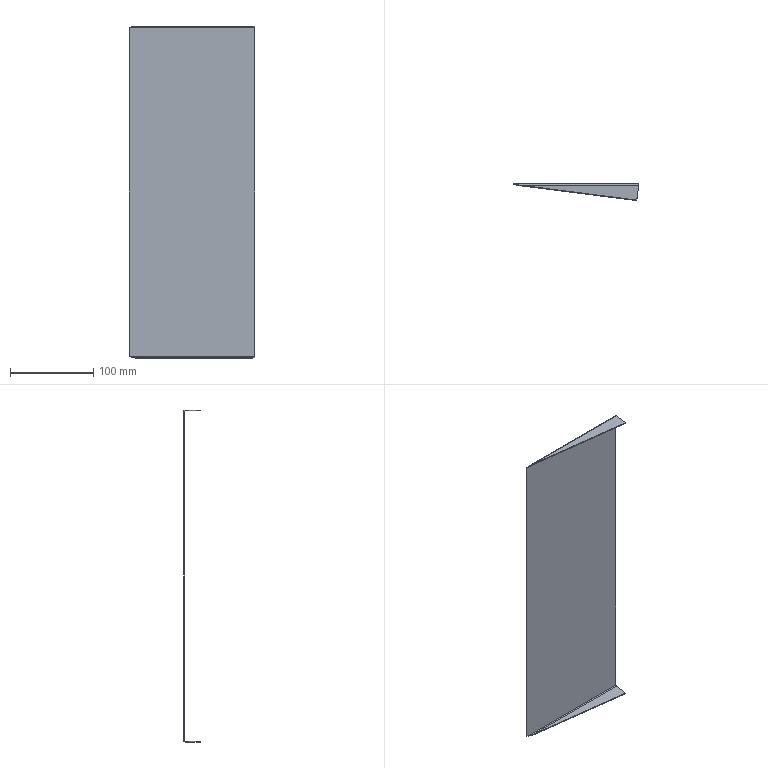Part | SolidWorks | features EdgeFlange 1, FlatPattern 1, MirrorPattern 1, SMBaseFlange 1, SheetMetal 1 | 1 solid | 20 faces | box 151 x 20 x 399 mm | volume 62913 mm3 | plane 12 | spline 4 | cylinder 4 | commonest cylinder face diameters 2 x2 4 x2
STEP:
#1=CARTESIAN_POINT('',(0.,-1.,-197.5));
#2=VERTEX_POINT('',#1);
#3=CARTESIAN_POINT('',(-151.,-1.,-197.5));
#4=VERTEX_POINT('',#3);
#5=CARTESIAN_POINT('',(0.,-1.,-197.5));
#6=DIRECTION('',(-1.,0.,0.));
#7=VECTOR('',#6,1000.);
#8=LINE('',#5,#7);
#9=EDGE_CURVE('',#2,#4,#8,.T.);
#10=ORIENTED_EDGE('',*,*,#9,.F.);
#11=CARTESIAN_POINT('',(0.,-1.,197.5));
#12=VERTEX_POINT('',#11);
#13=CARTESIAN_POINT('',(0.,-1.,199.5));
#14=DIRECTION('',(0.,0.,-1.));
#15=VECTOR('',#14,1000.);
#16=LINE('',#13,#15);
#17=EDGE_CURVE('',#12,#2,#16,.T.);
#18=ORIENTED_EDGE('',*,*,#17,.F.);
#19=CARTESIAN_POINT('',(-151.,-1.,197.5));
#20=VERTEX_POINT('',#19);
#21=CARTESIAN_POINT('',(-151.,-1.,197.5));
#22=DIRECTION('',(1.,0.,0.));
#23=VECTOR('',#22,1000.);
#24=LINE('',#21,#23);
#25=EDGE_CURVE('',#20,#12,#24,.T.);
#26=ORIENTED_EDGE('',*,*,#25,.F.);
#27=CARTESIAN_POINT('',(-151.,-1.,199.5));
#28=DIRECTION('',(0.,0.,-1.));
#29=VECTOR('',#28,1000.);
#30=LINE('',#27,#29);
#31=EDGE_CURVE('',#20,#4,#30,.T.);
#32=ORIENTED_EDGE('',*,*,#31,.T.);
#33=EDGE_LOOP('',(#10,#18,#26,#32));
#34=FACE_OUTER_BOUND('',#33,.T.);
#35=CARTESIAN_POINT('',(-151.,-1.,199.5));
#36=DIRECTION('',(0.,1.,0.));
#37=DIRECTION('',(0.,0.,1.));
#38=AXIS2_PLACEMENT_3D('',#35,#36,#37);
#39=PLANE('',#38);
#40=ADVANCED_FACE('',(#34),#39,.F.);
#41=CARTESIAN_POINT('',(0.,0.,197.5));
#42=VERTEX_POINT('',#41);
#43=CARTESIAN_POINT('',(0.,0.,-197.5));
#44=VERTEX_POINT('',#43);
#45=CARTESIAN_POINT('',(0.,0.,199.5));
#46=DIRECTION('',(0.,0.,-1.));
#47=VECTOR('',#46,1000.);
#48=LINE('',#45,#47);
#49=EDGE_CURVE('',#42,#44,#48,.T.);
#50=ORIENTED_EDGE('',*,*,#49,.T.);
#51=CARTESIAN_POINT('',(-151.,0.,-197.5));
#52=VERTEX_POINT('',#51);
#53=CARTESIAN_POINT('',(0.,0.,-197.5));
#54=DIRECTION('',(-1.,0.,0.));
#55=VECTOR('',#54,1000.);
#56=LINE('',#53,#55);
#57=EDGE_CURVE('',#44,#52,#56,.T.);
#58=ORIENTED_EDGE('',*,*,#57,.T.);
#59=CARTESIAN_POINT('',(-151.,0.,197.5));
#60=VERTEX_POINT('',#59);
#61=CARTESIAN_POINT('',(-151.,0.,199.5));
#62=DIRECTION('',(0.,0.,-1.));
#63=VECTOR('',#62,1000.);
#64=LINE('',#61,#63);
#65=EDGE_CURVE('',#60,#52,#64,.T.);
#66=ORIENTED_EDGE('',*,*,#65,.F.);
#67=CARTESIAN_POINT('',(-151.,0.,197.5));
#68=DIRECTION('',(1.,0.,0.));
#69=VECTOR('',#68,1000.);
#70=LINE('',#67,#69);
#71=EDGE_CURVE('',#60,#42,#70,.T.);
#72=ORIENTED_EDGE('',*,*,#71,.T.);
#73=EDGE_LOOP('',(#50,#58,#66,#72));
#74=FACE_OUTER_BOUND('',#73,.T.);
#75=CARTESIAN_POINT('',(-151.,0.,199.5));
#76=DIRECTION('',(0.,1.,0.));
#77=DIRECTION('',(0.,0.,1.));
#78=AXIS2_PLACEMENT_3D('',#75,#76,#77);
#79=PLANE('',#78);
#80=ADVANCED_FACE('',(#74),#79,.T.);
#81=ORIENTED_EDGE('',*,*,#17,.T.);
#82=CARTESIAN_POINT('',(0.,-1.,-197.5));
#83=DIRECTION('',(0.,1.,0.));
#84=VECTOR('',#83,1000.);
#85=LINE('',#82,#84);
#86=EDGE_CURVE('',#2,#44,#85,.T.);
#87=ORIENTED_EDGE('',*,*,#86,.T.);
#88=ORIENTED_EDGE('',*,*,#49,.F.);
#89=CARTESIAN_POINT('',(0.,-1.,197.5));
#90=DIRECTION('',(0.,1.,0.));
#91=VECTOR('',#90,1000.);
#92=LINE('',#89,#91);
#93=EDGE_CURVE('',#12,#42,#92,.T.);
#94=ORIENTED_EDGE('',*,*,#93,.F.);
#95=EDGE_LOOP('',(#81,#87,#88,#94));
#96=FACE_OUTER_BOUND('',#95,.T.);
#97=CARTESIAN_POINT('',(0.,0.,199.5));
#98=DIRECTION('',(1.,0.,0.));
#99=DIRECTION('',(0.,0.,-1.));
#100=AXIS2_PLACEMENT_3D('',#97,#98,#99);
#101=PLANE('',#100);
#102=ADVANCED_FACE('',(#96),#101,.T.);
#103=CARTESIAN_POINT('',(-151.,-1.,-197.5));
#104=DIRECTION('',(0.,1.,0.));
#105=VECTOR('',#104,1000.);
#106=LINE('',#103,#105);
#107=EDGE_CURVE('',#4,#52,#106,.T.);
#108=ORIENTED_EDGE('',*,*,#107,.F.);
#109=ORIENTED_EDGE('',*,*,#31,.F.);
#110=CARTESIAN_POINT('',(-151.,-1.,197.5));
#111=DIRECTION('',(0.,1.,0.));
#112=VECTOR('',#111,1000.);
#113=LINE('',#110,#112);
#114=EDGE_CURVE('',#20,#60,#113,.T.);
#115=ORIENTED_EDGE('',*,*,#114,.T.);
#116=ORIENTED_EDGE('',*,*,#65,.T.);
#117=EDGE_LOOP('',(#108,#109,#115,#116));
#118=FACE_OUTER_BOUND('',#117,.T.);
#119=CARTESIAN_POINT('',(-151.,-1.,199.5));
#120=DIRECTION('',(-1.,0.,0.));
#121=DIRECTION('',(0.,0.,1.));
#122=AXIS2_PLACEMENT_3D('',#119,#120,#121);
#123=PLANE('',#122);
#124=ADVANCED_FACE('',(#118),#123,.T.);
#125=CARTESIAN_POINT('',(-0.1279,-2.,198.5));
#126=VERTEX_POINT('',#125);
#127=CARTESIAN_POINT('',(-0.1279,-2.,199.5));
#128=VERTEX_POINT('',#127);
#129=CARTESIAN_POINT('',(-0.1279,-2.,199.5));
#130=DIRECTION('',(0.,0.,1.));
#131=VECTOR('',#130,1000.);
#132=LINE('',#129,#131);
#133=EDGE_CURVE('',#126,#128,#132,.T.);
#134=ORIENTED_EDGE('',*,*,#133,.F.);
#135=CARTESIAN_POINT('',(0.,-1.,197.5));
#136=CARTESIAN_POINT('',(-0.02131,-1.,197.762));
#137=CARTESIAN_POINT('',(-0.04263,-1.108,198.022));
#138=CARTESIAN_POINT('',(-0.08526,-1.478,198.392));
#139=CARTESIAN_POINT('',(-0.1066,-1.738,198.5));
#140=CARTESIAN_POINT('',(-0.1279,-2.,198.5));
#141=B_SPLINE_CURVE_WITH_KNOTS('',3,(#135,#136,#137,#138,#139,#140),.UNSPECIFIED.,.F.,.F.,(4,2,4),(0.,0.5,1.),.UNSPECIFIED.);
#142=EDGE_CURVE('',#12,#126,#141,.T.);
#143=ORIENTED_EDGE('',*,*,#142,.F.);
#144=ORIENTED_EDGE('',*,*,#93,.T.);
#145=CARTESIAN_POINT('',(0.,0.,197.5));
#146=CARTESIAN_POINT('',(-0.01066,0.,197.762));
#147=CARTESIAN_POINT('',(-0.02131,-0.05205,198.023));
#148=CARTESIAN_POINT('',(-0.04263,-0.2524,198.507));
#149=CARTESIAN_POINT('',(-0.05329,-0.4007,198.729));
#150=CARTESIAN_POINT('',(-0.0746,-0.7709,199.099));
#151=CARTESIAN_POINT('',(-0.08526,-0.9928,199.248));
#152=CARTESIAN_POINT('',(-0.1066,-1.477,199.448));
#153=CARTESIAN_POINT('',(-0.1172,-1.738,199.5));
#154=CARTESIAN_POINT('',(-0.1279,-2.,199.5));
#155=B_SPLINE_CURVE_WITH_KNOTS('',3,(#145,#146,#147,#148,#149,#150,#151,#152,#153,#154),.UNSPECIFIED.,.F.,.F.,(4,2,2,2,4),(0.,0.25,0.5,0.75,1.),.UNSPECIFIED.);
#156=EDGE_CURVE('',#42,#128,#155,.T.);
#157=ORIENTED_EDGE('',*,*,#156,.T.);
#158=EDGE_LOOP('',(#134,#143,#144,#157));
#159=FACE_OUTER_BOUND('',#158,.T.);
#160=CARTESIAN_POINT('',(0.,0.01,197.5));
#161=CARTESIAN_POINT('',(-0.01066,0.01,197.763));
#162=CARTESIAN_POINT('',(-0.02131,-0.04231,198.026));
#163=CARTESIAN_POINT('',(-0.04263,-0.2437,198.512));
#164=CARTESIAN_POINT('',(-0.05329,-0.3927,198.735));
#165=CARTESIAN_POINT('',(-0.0746,-0.7648,199.107));
#166=CARTESIAN_POINT('',(-0.08526,-0.9877,199.256));
#167=CARTESIAN_POINT('',(-0.1066,-1.474,199.458));
#168=CARTESIAN_POINT('',(-0.1172,-1.737,199.51));
#169=CARTESIAN_POINT('',(-0.1279,-2.,199.51));
#170=CARTESIAN_POINT('',(0.,0.,197.5));
#171=CARTESIAN_POINT('',(-0.01066,0.,197.762));
#172=CARTESIAN_POINT('',(-0.02131,-0.05205,198.023));
#173=CARTESIAN_POINT('',(-0.04263,-0.2524,198.507));
#174=CARTESIAN_POINT('',(-0.05329,-0.4007,198.729));
#175=CARTESIAN_POINT('',(-0.0746,-0.7709,199.099));
#176=CARTESIAN_POINT('',(-0.08526,-0.9928,199.248));
#177=CARTESIAN_POINT('',(-0.1066,-1.477,199.448));
#178=CARTESIAN_POINT('',(-0.1172,-1.738,199.5));
#179=CARTESIAN_POINT('',(-0.1279,-2.,199.5));
#180=CARTESIAN_POINT('',(0.,-1.,197.5));
#181=CARTESIAN_POINT('',(-0.01066,-1.,197.631));
#182=CARTESIAN_POINT('',(-0.02131,-1.026,197.762));
#183=CARTESIAN_POINT('',(-0.04263,-1.126,198.004));
#184=CARTESIAN_POINT('',(-0.05329,-1.2,198.115));
#185=CARTESIAN_POINT('',(-0.0746,-1.385,198.3));
#186=CARTESIAN_POINT('',(-0.08526,-1.496,198.374));
#187=CARTESIAN_POINT('',(-0.1066,-1.738,198.474));
#188=CARTESIAN_POINT('',(-0.1172,-1.869,198.5));
#189=CARTESIAN_POINT('',(-0.1279,-2.,198.5));
#190=CARTESIAN_POINT('',(0.,-1.01,197.5));
#191=CARTESIAN_POINT('',(-0.01066,-1.01,197.63));
#192=CARTESIAN_POINT('',(-0.02131,-1.036,197.759));
#193=CARTESIAN_POINT('',(-0.04263,-1.135,197.999));
#194=CARTESIAN_POINT('',(-0.05329,-1.208,198.108));
#195=CARTESIAN_POINT('',(-0.0746,-1.392,198.292));
#196=CARTESIAN_POINT('',(-0.08526,-1.501,198.365));
#197=CARTESIAN_POINT('',(-0.1066,-1.741,198.464));
#198=CARTESIAN_POINT('',(-0.1172,-1.87,198.49));
#199=CARTESIAN_POINT('',(-0.1279,-2.,198.49));
#200=B_SPLINE_SURFACE_WITH_KNOTS('',1,3,((#160,#161,#162,#163,#164,#165,#166,#167,#168,#169),(#170,#171,#172,#173,#174,#175,#176,#177,#178,#179),(#180,#181,#182,#183,#184,#185,#186,#187,#188,#189),(#190,#191,#192,#193,#194,#195,#196,#197,#198,#199)),.UNSPECIFIED.,.F.,.F.,.F.,(2,1,1,2),(4,2,2,2,4),(-0.01,0.,1.,1.01),(0.,0.25,0.5,0.75,1.),.UNSPECIFIED.);
#201=ADVANCED_FACE('',(#159),#200,.F.);
#202=CARTESIAN_POINT('',(-143.181,-2.,198.5));
#203=VERTEX_POINT('',#202);
#204=CARTESIAN_POINT('',(-143.181,-2.,198.5));
#205=CARTESIAN_POINT('',(-144.485,-1.738,198.5));
#206=CARTESIAN_POINT('',(-145.788,-1.478,198.392));
#207=CARTESIAN_POINT('',(-148.398,-1.107,198.021));
#208=CARTESIAN_POINT('',(-149.695,-1.,197.762));
#209=CARTESIAN_POINT('',(-151.,-1.,197.5));
#210=B_SPLINE_CURVE_WITH_KNOTS('',3,(#204,#205,#206,#207,#208,#209),.UNSPECIFIED.,.F.,.F.,(4,2,4),(0.,0.00399,0.007979),.UNSPECIFIED.);
#211=EDGE_CURVE('',#203,#20,#210,.T.);
#212=ORIENTED_EDGE('',*,*,#211,.F.);
#213=CARTESIAN_POINT('',(-143.181,-2.,199.5));
#214=VERTEX_POINT('',#213);
#215=CARTESIAN_POINT('',(-143.181,-2.,198.5));
#216=DIRECTION('',(0.,0.,1.));
#217=VECTOR('',#216,1000.);
#218=LINE('',#215,#217);
#219=EDGE_CURVE('',#203,#214,#218,.T.);
#220=ORIENTED_EDGE('',*,*,#219,.T.);
#221=CARTESIAN_POINT('',(-143.181,-2.,199.5));
#222=CARTESIAN_POINT('',(-143.835,-1.737,199.5));
#223=CARTESIAN_POINT('',(-144.487,-1.475,199.448));
#224=CARTESIAN_POINT('',(-145.794,-0.9902,199.246));
#225=CARTESIAN_POINT('',(-146.442,-0.7701,199.098));
#226=CARTESIAN_POINT('',(-147.738,-0.4018,198.73));
#227=CARTESIAN_POINT('',(-148.388,-0.2535,198.509));
#228=CARTESIAN_POINT('',(-149.695,-0.05212,198.024));
#229=CARTESIAN_POINT('',(-150.346,0.,197.763));
#230=CARTESIAN_POINT('',(-151.,0.,197.5));
#231=B_SPLINE_CURVE_WITH_KNOTS('',3,(#221,#222,#223,#224,#225,#226,#227,#228,#229,#230),.UNSPECIFIED.,.F.,.F.,(4,2,2,2,4),(0.,0.00211,0.004221,0.006331,0.008441),.UNSPECIFIED.);
#232=EDGE_CURVE('',#214,#60,#231,.T.);
#233=ORIENTED_EDGE('',*,*,#232,.T.);
#234=ORIENTED_EDGE('',*,*,#114,.F.);
#235=EDGE_LOOP('',(#212,#220,#233,#234));
#236=FACE_OUTER_BOUND('',#235,.T.);
#237=CARTESIAN_POINT('',(-143.181,-2.,199.51));
#238=CARTESIAN_POINT('',(-143.832,-1.737,199.51));
#239=CARTESIAN_POINT('',(-144.484,-1.474,199.458));
#240=CARTESIAN_POINT('',(-145.787,-0.9877,199.256));
#241=CARTESIAN_POINT('',(-146.439,-0.7648,199.107));
#242=CARTESIAN_POINT('',(-147.742,-0.3927,198.735));
#243=CARTESIAN_POINT('',(-148.394,-0.2437,198.512));
#244=CARTESIAN_POINT('',(-149.697,-0.04231,198.026));
#245=CARTESIAN_POINT('',(-150.348,0.01,197.763));
#246=CARTESIAN_POINT('',(-151.,0.01,197.5));
#247=CARTESIAN_POINT('',(-143.181,-2.,199.5));
#248=CARTESIAN_POINT('',(-143.832,-1.738,199.5));
#249=CARTESIAN_POINT('',(-144.484,-1.477,199.448));
#250=CARTESIAN_POINT('',(-145.787,-0.9928,199.248));
#251=CARTESIAN_POINT('',(-146.439,-0.7709,199.099));
#252=CARTESIAN_POINT('',(-147.742,-0.4007,198.729));
#253=CARTESIAN_POINT('',(-148.394,-0.2524,198.507));
#254=CARTESIAN_POINT('',(-149.697,-0.05205,198.023));
#255=CARTESIAN_POINT('',(-150.348,0.,197.762));
#256=CARTESIAN_POINT('',(-151.,0.,197.5));
#257=CARTESIAN_POINT('',(-143.181,-2.,198.5));
#258=CARTESIAN_POINT('',(-143.832,-1.869,198.5));
#259=CARTESIAN_POINT('',(-144.484,-1.738,198.474));
#260=CARTESIAN_POINT('',(-145.787,-1.496,198.374));
#261=CARTESIAN_POINT('',(-146.439,-1.385,198.3));
#262=CARTESIAN_POINT('',(-147.742,-1.2,198.115));
#263=CARTESIAN_POINT('',(-148.394,-1.126,198.004));
#264=CARTESIAN_POINT('',(-149.697,-1.026,197.762));
#265=CARTESIAN_POINT('',(-150.348,-1.,197.631));
#266=CARTESIAN_POINT('',(-151.,-1.,197.5));
#267=CARTESIAN_POINT('',(-143.181,-2.,198.49));
#268=CARTESIAN_POINT('',(-143.832,-1.87,198.49));
#269=CARTESIAN_POINT('',(-144.484,-1.741,198.464));
#270=CARTESIAN_POINT('',(-145.787,-1.501,198.365));
#271=CARTESIAN_POINT('',(-146.439,-1.392,198.292));
#272=CARTESIAN_POINT('',(-147.742,-1.208,198.108));
#273=CARTESIAN_POINT('',(-148.394,-1.135,197.999));
#274=CARTESIAN_POINT('',(-149.697,-1.036,197.759));
#275=CARTESIAN_POINT('',(-150.348,-1.01,197.63));
#276=CARTESIAN_POINT('',(-151.,-1.01,197.5));
#277=B_SPLINE_SURFACE_WITH_KNOTS('',1,3,((#237,#238,#239,#240,#241,#242,#243,#244,#245,#246),(#247,#248,#249,#250,#251,#252,#253,#254,#255,#256),(#257,#258,#259,#260,#261,#262,#263,#264,#265,#266),(#267,#268,#269,#270,#271,#272,#273,#274,#275,#276)),.UNSPECIFIED.,.F.,.F.,.F.,(2,1,1,2),(4,2,2,2,4),(-0.01,0.,1.,1.01),(0.,0.25,0.5,0.75,1.),.UNSPECIFIED.);
#278=ADVANCED_FACE('',(#236),#277,.F.);
#279=ORIENTED_EDGE('',*,*,#71,.F.);
#280=ORIENTED_EDGE('',*,*,#232,.F.);
#281=CARTESIAN_POINT('',(-0.1279,-2.,199.5));
#282=DIRECTION('',(1.,0.,0.));
#283=VECTOR('',#282,1000.);
#284=LINE('',#281,#283);
#285=EDGE_CURVE('',#214,#128,#284,.T.);
#286=ORIENTED_EDGE('',*,*,#285,.T.);
#287=ORIENTED_EDGE('',*,*,#156,.F.);
#288=EDGE_LOOP('',(#279,#280,#286,#287));
#289=FACE_OUTER_BOUND('',#288,.T.);
#290=CARTESIAN_POINT('',(-151.,-2.,197.5));
#291=DIRECTION('',(-1.,0.,0.));
#292=DIRECTION('',(0.,0.,1.));
#293=AXIS2_PLACEMENT_3D('',#290,#291,#292);
#294=CYLINDRICAL_SURFACE('',#293,2.);
#295=ADVANCED_FACE('',(#289),#294,.T.);
#296=ORIENTED_EDGE('',*,*,#25,.T.);
#297=ORIENTED_EDGE('',*,*,#142,.T.);
#298=CARTESIAN_POINT('',(-0.1279,-2.,198.5));
#299=DIRECTION('',(-1.,0.,0.));
#300=VECTOR('',#299,1000.);
#301=LINE('',#298,#300);
#302=EDGE_CURVE('',#126,#203,#301,.T.);
#303=ORIENTED_EDGE('',*,*,#302,.T.);
#304=ORIENTED_EDGE('',*,*,#211,.T.);
#305=EDGE_LOOP('',(#296,#297,#303,#304));
#306=FACE_OUTER_BOUND('',#305,.T.);
#307=CARTESIAN_POINT('',(-151.,-2.,197.5));
#308=DIRECTION('',(-1.,0.,0.));
#309=DIRECTION('',(0.,0.,1.));
#310=AXIS2_PLACEMENT_3D('',#307,#308,#309);
#311=CYLINDRICAL_SURFACE('',#310,1.);
#312=ADVANCED_FACE('',(#306),#311,.F.);
#313=CARTESIAN_POINT('',(-2.43,-20.,199.5));
#314=VERTEX_POINT('',#313);
#315=CARTESIAN_POINT('',(-151.,-1.,199.5));
#316=DIRECTION('',(-0.9919,0.1269,0.));
#317=VECTOR('',#316,1000.);
#318=LINE('',#315,#317);
#319=EDGE_CURVE('',#314,#214,#318,.T.);
#320=ORIENTED_EDGE('',*,*,#319,.T.);
#321=ORIENTED_EDGE('',*,*,#219,.F.);
#322=CARTESIAN_POINT('',(-2.43,-20.,198.5));
#323=VERTEX_POINT('',#322);
#324=CARTESIAN_POINT('',(-2.556,-19.984,198.5));
#325=DIRECTION('',(-0.9919,0.1269,0.));
#326=VECTOR('',#325,1000.);
#327=LINE('',#324,#326);
#328=EDGE_CURVE('',#323,#203,#327,.T.);
#329=ORIENTED_EDGE('',*,*,#328,.F.);
#330=CARTESIAN_POINT('',(-2.43,-20.,199.5));
#331=DIRECTION('',(0.,0.,-1.));
#332=VECTOR('',#331,1000.);
#333=LINE('',#330,#332);
#334=EDGE_CURVE('',#314,#323,#333,.T.);
#335=ORIENTED_EDGE('',*,*,#334,.F.);
#336=EDGE_LOOP('',(#320,#321,#329,#335));
#337=FACE_OUTER_BOUND('',#336,.T.);
#338=CARTESIAN_POINT('',(-151.,-1.,199.5));
#339=DIRECTION('',(-0.1269,-0.9919,0.));
#340=DIRECTION('',(0.9919,-0.1269,0.));
#341=AXIS2_PLACEMENT_3D('',#338,#339,#340);
#342=PLANE('',#341);
#343=ADVANCED_FACE('',(#337),#342,.T.);
#344=CARTESIAN_POINT('',(0.1258,-0.01609,198.5));
#345=DIRECTION('',(-0.1269,-0.9919,0.));
#346=VECTOR('',#345,1000.);
#347=LINE('',#344,#346);
#348=EDGE_CURVE('',#126,#323,#347,.T.);
#349=ORIENTED_EDGE('',*,*,#348,.F.);
#350=ORIENTED_EDGE('',*,*,#133,.T.);
#351=CARTESIAN_POINT('',(-2.43,-20.,199.5));
#352=DIRECTION('',(-0.1269,-0.9919,0.));
#353=VECTOR('',#352,1000.);
#354=LINE('',#351,#353);
#355=EDGE_CURVE('',#128,#314,#354,.T.);
#356=ORIENTED_EDGE('',*,*,#355,.T.);
#357=ORIENTED_EDGE('',*,*,#334,.T.);
#358=EDGE_LOOP('',(#349,#350,#356,#357));
#359=FACE_OUTER_BOUND('',#358,.T.);
#360=CARTESIAN_POINT('',(-2.43,-20.,199.5));
#361=DIRECTION('',(0.9919,-0.1269,0.));
#362=DIRECTION('',(0.1269,0.9919,0.));
#363=AXIS2_PLACEMENT_3D('',#360,#361,#362);
#364=PLANE('',#363);
#365=ADVANCED_FACE('',(#359),#364,.T.);
#366=ORIENTED_EDGE('',*,*,#285,.F.);
#367=ORIENTED_EDGE('',*,*,#319,.F.);
#368=ORIENTED_EDGE('',*,*,#355,.F.);
#369=EDGE_LOOP('',(#366,#367,#368));
#370=FACE_OUTER_BOUND('',#369,.T.);
#371=CARTESIAN_POINT('',(0.,0.,199.5));
#372=DIRECTION('',(0.,0.,-1.));
#373=DIRECTION('',(0.,1.,0.));
#374=AXIS2_PLACEMENT_3D('',#371,#372,#373);
#375=PLANE('',#374);
#376=ADVANCED_FACE('',(#370),#375,.F.);
#377=ORIENTED_EDGE('',*,*,#328,.T.);
#378=ORIENTED_EDGE('',*,*,#302,.F.);
#379=ORIENTED_EDGE('',*,*,#348,.T.);
#380=EDGE_LOOP('',(#377,#378,#379));
#381=FACE_OUTER_BOUND('',#380,.T.);
#382=CARTESIAN_POINT('',(0.,0.,198.5));
#383=DIRECTION('',(0.,0.,-1.));
#384=DIRECTION('',(0.,1.,0.));
#385=AXIS2_PLACEMENT_3D('',#382,#383,#384);
#386=PLANE('',#385);
#387=ADVANCED_FACE('',(#381),#386,.T.);
#388=CARTESIAN_POINT('',(-143.181,-2.,-198.5));
#389=VERTEX_POINT('',#388);
#390=CARTESIAN_POINT('',(-143.181,-2.,-199.5));
#391=VERTEX_POINT('',#390);
#392=CARTESIAN_POINT('',(-143.181,-2.,-199.5));
#393=DIRECTION('',(0.,0.,-1.));
#394=VECTOR('',#393,1000.);
#395=LINE('',#392,#394);
#396=EDGE_CURVE('',#389,#391,#395,.T.);
#397=ORIENTED_EDGE('',*,*,#396,.F.);
#398=CARTESIAN_POINT('',(-151.,-1.,-197.5));
#399=CARTESIAN_POINT('',(-149.695,-1.,-197.762));
#400=CARTESIAN_POINT('',(-148.392,-1.108,-198.022));
#401=CARTESIAN_POINT('',(-145.783,-1.479,-198.393));
#402=CARTESIAN_POINT('',(-144.485,-1.738,-198.5));
#403=CARTESIAN_POINT('',(-143.181,-2.,-198.5));
#404=B_SPLINE_CURVE_WITH_KNOTS('',3,(#398,#399,#400,#401,#402,#403),.UNSPECIFIED.,.F.,.F.,(4,2,4),(0.,0.00399,0.007979),.UNSPECIFIED.);
#405=EDGE_CURVE('',#4,#389,#404,.T.);
#406=ORIENTED_EDGE('',*,*,#405,.F.);
#407=ORIENTED_EDGE('',*,*,#107,.T.);
#408=CARTESIAN_POINT('',(-151.,0.,-197.5));
#409=CARTESIAN_POINT('',(-150.346,0.,-197.763));
#410=CARTESIAN_POINT('',(-149.694,-0.05225,-198.025));
#411=CARTESIAN_POINT('',(-148.386,-0.2538,-198.51));
#412=CARTESIAN_POINT('',(-147.739,-0.4016,-198.73));
#413=CARTESIAN_POINT('',(-146.443,-0.7697,-199.098));
#414=CARTESIAN_POINT('',(-145.793,-0.9907,-199.247));
#415=CARTESIAN_POINT('',(-144.485,-1.476,-199.448));
#416=CARTESIAN_POINT('',(-143.835,-1.737,-199.5));
#417=CARTESIAN_POINT('',(-143.181,-2.,-199.5));
#418=B_SPLINE_CURVE_WITH_KNOTS('',3,(#408,#409,#410,#411,#412,#413,#414,#415,#416,#417),.UNSPECIFIED.,.F.,.F.,(4,2,2,2,4),(0.,0.00211,0.004221,0.006331,0.008441),.UNSPECIFIED.);
#419=EDGE_CURVE('',#52,#391,#418,.T.);
#420=ORIENTED_EDGE('',*,*,#419,.T.);
#421=EDGE_LOOP('',(#397,#406,#407,#420));
#422=FACE_OUTER_BOUND('',#421,.T.);
#423=CARTESIAN_POINT('',(-151.,0.01,-197.5));
#424=CARTESIAN_POINT('',(-150.348,0.01,-197.763));
#425=CARTESIAN_POINT('',(-149.697,-0.04231,-198.026));
#426=CARTESIAN_POINT('',(-148.394,-0.2437,-198.512));
#427=CARTESIAN_POINT('',(-147.742,-0.3927,-198.735));
#428=CARTESIAN_POINT('',(-146.439,-0.7648,-199.107));
#429=CARTESIAN_POINT('',(-145.787,-0.9877,-199.256));
#430=CARTESIAN_POINT('',(-144.484,-1.474,-199.458));
#431=CARTESIAN_POINT('',(-143.832,-1.737,-199.51));
#432=CARTESIAN_POINT('',(-143.181,-2.,-199.51));
#433=CARTESIAN_POINT('',(-151.,0.,-197.5));
#434=CARTESIAN_POINT('',(-150.348,0.,-197.762));
#435=CARTESIAN_POINT('',(-149.697,-0.05205,-198.023));
#436=CARTESIAN_POINT('',(-148.394,-0.2524,-198.507));
#437=CARTESIAN_POINT('',(-147.742,-0.4007,-198.729));
#438=CARTESIAN_POINT('',(-146.439,-0.7709,-199.099));
#439=CARTESIAN_POINT('',(-145.787,-0.9928,-199.248));
#440=CARTESIAN_POINT('',(-144.484,-1.477,-199.448));
#441=CARTESIAN_POINT('',(-143.832,-1.738,-199.5));
#442=CARTESIAN_POINT('',(-143.181,-2.,-199.5));
#443=CARTESIAN_POINT('',(-151.,-1.,-197.5));
#444=CARTESIAN_POINT('',(-150.348,-1.,-197.631));
#445=CARTESIAN_POINT('',(-149.697,-1.026,-197.762));
#446=CARTESIAN_POINT('',(-148.394,-1.126,-198.004));
#447=CARTESIAN_POINT('',(-147.742,-1.2,-198.115));
#448=CARTESIAN_POINT('',(-146.439,-1.385,-198.3));
#449=CARTESIAN_POINT('',(-145.787,-1.496,-198.374));
#450=CARTESIAN_POINT('',(-144.484,-1.738,-198.474));
#451=CARTESIAN_POINT('',(-143.832,-1.869,-198.5));
#452=CARTESIAN_POINT('',(-143.181,-2.,-198.5));
#453=CARTESIAN_POINT('',(-151.,-1.01,-197.5));
#454=CARTESIAN_POINT('',(-150.348,-1.01,-197.63));
#455=CARTESIAN_POINT('',(-149.697,-1.036,-197.759));
#456=CARTESIAN_POINT('',(-148.394,-1.135,-197.999));
#457=CARTESIAN_POINT('',(-147.742,-1.208,-198.108));
#458=CARTESIAN_POINT('',(-146.439,-1.392,-198.292));
#459=CARTESIAN_POINT('',(-145.787,-1.501,-198.365));
#460=CARTESIAN_POINT('',(-144.484,-1.741,-198.464));
#461=CARTESIAN_POINT('',(-143.832,-1.87,-198.49));
#462=CARTESIAN_POINT('',(-143.181,-2.,-198.49));
#463=B_SPLINE_SURFACE_WITH_KNOTS('',1,3,((#423,#424,#425,#426,#427,#428,#429,#430,#431,#432),(#433,#434,#435,#436,#437,#438,#439,#440,#441,#442),(#443,#444,#445,#446,#447,#448,#449,#450,#451,#452),(#453,#454,#455,#456,#457,#458,#459,#460,#461,#462)),.UNSPECIFIED.,.F.,.F.,.F.,(2,1,1,2),(4,2,2,2,4),(-0.01,0.,1.,1.01),(0.,0.25,0.5,0.75,1.),.UNSPECIFIED.);
#464=ADVANCED_FACE('',(#422),#463,.F.);
#465=CARTESIAN_POINT('',(-0.1279,-2.,-198.5));
#466=VERTEX_POINT('',#465);
#467=CARTESIAN_POINT('',(-0.1279,-2.,-198.5));
#468=CARTESIAN_POINT('',(-0.1066,-1.738,-198.5));
#469=CARTESIAN_POINT('',(-0.08526,-1.478,-198.392));
#470=CARTESIAN_POINT('',(-0.04263,-1.108,-198.022));
#471=CARTESIAN_POINT('',(-0.02131,-1.,-197.762));
#472=CARTESIAN_POINT('',(0.,-1.,-197.5));
#473=B_SPLINE_CURVE_WITH_KNOTS('',3,(#467,#468,#469,#470,#471,#472),.UNSPECIFIED.,.F.,.F.,(4,2,4),(0.,0.5,1.),.UNSPECIFIED.);
#474=EDGE_CURVE('',#466,#2,#473,.T.);
#475=ORIENTED_EDGE('',*,*,#474,.F.);
#476=CARTESIAN_POINT('',(-0.1279,-2.,-199.5));
#477=VERTEX_POINT('',#476);
#478=CARTESIAN_POINT('',(-0.1279,-2.,-198.5));
#479=DIRECTION('',(0.,0.,-1.));
#480=VECTOR('',#479,1000.);
#481=LINE('',#478,#480);
#482=EDGE_CURVE('',#466,#477,#481,.T.);
#483=ORIENTED_EDGE('',*,*,#482,.T.);
#484=CARTESIAN_POINT('',(-0.1279,-2.,-199.5));
#485=CARTESIAN_POINT('',(-0.1172,-1.738,-199.5));
#486=CARTESIAN_POINT('',(-0.1066,-1.477,-199.448));
#487=CARTESIAN_POINT('',(-0.08526,-0.9928,-199.248));
#488=CARTESIAN_POINT('',(-0.0746,-0.7709,-199.099));
#489=CARTESIAN_POINT('',(-0.05329,-0.4007,-198.729));
#490=CARTESIAN_POINT('',(-0.04263,-0.2524,-198.507));
#491=CARTESIAN_POINT('',(-0.02131,-0.05205,-198.023));
#492=CARTESIAN_POINT('',(-0.01066,0.,-197.762));
#493=CARTESIAN_POINT('',(0.,0.,-197.5));
#494=B_SPLINE_CURVE_WITH_KNOTS('',3,(#484,#485,#486,#487,#488,#489,#490,#491,#492,#493),.UNSPECIFIED.,.F.,.F.,(4,2,2,2,4),(0.,0.25,0.5,0.75,1.),.UNSPECIFIED.);
#495=EDGE_CURVE('',#477,#44,#494,.T.);
#496=ORIENTED_EDGE('',*,*,#495,.T.);
#497=ORIENTED_EDGE('',*,*,#86,.F.);
#498=EDGE_LOOP('',(#475,#483,#496,#497));
#499=FACE_OUTER_BOUND('',#498,.T.);
#500=CARTESIAN_POINT('',(-0.1279,-2.,-199.51));
#501=CARTESIAN_POINT('',(-0.1172,-1.737,-199.51));
#502=CARTESIAN_POINT('',(-0.1066,-1.474,-199.458));
#503=CARTESIAN_POINT('',(-0.08526,-0.9877,-199.256));
#504=CARTESIAN_POINT('',(-0.0746,-0.7648,-199.107));
#505=CARTESIAN_POINT('',(-0.05329,-0.3927,-198.735));
#506=CARTESIAN_POINT('',(-0.04263,-0.2437,-198.512));
#507=CARTESIAN_POINT('',(-0.02131,-0.04231,-198.026));
#508=CARTESIAN_POINT('',(-0.01066,0.01,-197.763));
#509=CARTESIAN_POINT('',(0.,0.01,-197.5));
#510=CARTESIAN_POINT('',(-0.1279,-2.,-199.5));
#511=CARTESIAN_POINT('',(-0.1172,-1.738,-199.5));
#512=CARTESIAN_POINT('',(-0.1066,-1.477,-199.448));
#513=CARTESIAN_POINT('',(-0.08526,-0.9928,-199.248));
#514=CARTESIAN_POINT('',(-0.0746,-0.7709,-199.099));
#515=CARTESIAN_POINT('',(-0.05329,-0.4007,-198.729));
#516=CARTESIAN_POINT('',(-0.04263,-0.2524,-198.507));
#517=CARTESIAN_POINT('',(-0.02131,-0.05205,-198.023));
#518=CARTESIAN_POINT('',(-0.01066,0.,-197.762));
#519=CARTESIAN_POINT('',(0.,0.,-197.5));
#520=CARTESIAN_POINT('',(-0.1279,-2.,-198.5));
#521=CARTESIAN_POINT('',(-0.1172,-1.869,-198.5));
#522=CARTESIAN_POINT('',(-0.1066,-1.738,-198.474));
#523=CARTESIAN_POINT('',(-0.08526,-1.496,-198.374));
#524=CARTESIAN_POINT('',(-0.0746,-1.385,-198.3));
#525=CARTESIAN_POINT('',(-0.05329,-1.2,-198.115));
#526=CARTESIAN_POINT('',(-0.04263,-1.126,-198.004));
#527=CARTESIAN_POINT('',(-0.02131,-1.026,-197.762));
#528=CARTESIAN_POINT('',(-0.01066,-1.,-197.631));
#529=CARTESIAN_POINT('',(0.,-1.,-197.5));
#530=CARTESIAN_POINT('',(-0.1279,-2.,-198.49));
#531=CARTESIAN_POINT('',(-0.1172,-1.87,-198.49));
#532=CARTESIAN_POINT('',(-0.1066,-1.741,-198.464));
#533=CARTESIAN_POINT('',(-0.08526,-1.501,-198.365));
#534=CARTESIAN_POINT('',(-0.0746,-1.392,-198.292));
#535=CARTESIAN_POINT('',(-0.05329,-1.208,-198.108));
#536=CARTESIAN_POINT('',(-0.04263,-1.135,-197.999));
#537=CARTESIAN_POINT('',(-0.02131,-1.036,-197.759));
#538=CARTESIAN_POINT('',(-0.01066,-1.01,-197.63));
#539=CARTESIAN_POINT('',(0.,-1.01,-197.5));
#540=B_SPLINE_SURFACE_WITH_KNOTS('',1,3,((#500,#501,#502,#503,#504,#505,#506,#507,#508,#509),(#510,#511,#512,#513,#514,#515,#516,#517,#518,#519),(#520,#521,#522,#523,#524,#525,#526,#527,#528,#529),(#530,#531,#532,#533,#534,#535,#536,#537,#538,#539)),.UNSPECIFIED.,.F.,.F.,.F.,(2,1,1,2),(4,2,2,2,4),(-0.01,0.,1.,1.01),(0.,0.25,0.5,0.75,1.),.UNSPECIFIED.);
#541=ADVANCED_FACE('',(#499),#540,.F.);
#542=ORIENTED_EDGE('',*,*,#57,.F.);
#543=ORIENTED_EDGE('',*,*,#495,.F.);
#544=CARTESIAN_POINT('',(-143.181,-2.,-199.5));
#545=DIRECTION('',(-1.,0.,0.));
#546=VECTOR('',#545,1000.);
#547=LINE('',#544,#546);
#548=EDGE_CURVE('',#477,#391,#547,.T.);
#549=ORIENTED_EDGE('',*,*,#548,.T.);
#550=ORIENTED_EDGE('',*,*,#419,.F.);
#551=EDGE_LOOP('',(#542,#543,#549,#550));
#552=FACE_OUTER_BOUND('',#551,.T.);
#553=CARTESIAN_POINT('',(0.,-2.,-197.5));
#554=DIRECTION('',(1.,0.,0.));
#555=DIRECTION('',(0.,0.,-1.));
#556=AXIS2_PLACEMENT_3D('',#553,#554,#555);
#557=CYLINDRICAL_SURFACE('',#556,2.);
#558=ADVANCED_FACE('',(#552),#557,.T.);
#559=ORIENTED_EDGE('',*,*,#9,.T.);
#560=ORIENTED_EDGE('',*,*,#405,.T.);
#561=CARTESIAN_POINT('',(-143.181,-2.,-198.5));
#562=DIRECTION('',(1.,0.,0.));
#563=VECTOR('',#562,1000.);
#564=LINE('',#561,#563);
#565=EDGE_CURVE('',#389,#466,#564,.T.);
#566=ORIENTED_EDGE('',*,*,#565,.T.);
#567=ORIENTED_EDGE('',*,*,#474,.T.);
#568=EDGE_LOOP('',(#559,#560,#566,#567));
#569=FACE_OUTER_BOUND('',#568,.T.);
#570=CARTESIAN_POINT('',(0.,-2.,-197.5));
#571=DIRECTION('',(1.,0.,0.));
#572=DIRECTION('',(0.,0.,-1.));
#573=AXIS2_PLACEMENT_3D('',#570,#571,#572);
#574=CYLINDRICAL_SURFACE('',#573,1.);
#575=ADVANCED_FACE('',(#569),#574,.F.);
#576=ORIENTED_EDGE('',*,*,#482,.F.);
#577=CARTESIAN_POINT('',(-2.43,-20.,-198.5));
#578=VERTEX_POINT('',#577);
#579=CARTESIAN_POINT('',(-2.43,-20.,-198.5));
#580=DIRECTION('',(-0.1269,-0.9919,0.));
#581=VECTOR('',#580,1000.);
#582=LINE('',#579,#581);
#583=EDGE_CURVE('',#466,#578,#582,.T.);
#584=ORIENTED_EDGE('',*,*,#583,.T.);
#585=CARTESIAN_POINT('',(-2.43,-20.,-199.5));
#586=VERTEX_POINT('',#585);
#587=CARTESIAN_POINT('',(-2.43,-20.,-199.5));
#588=DIRECTION('',(0.,0.,1.));
#589=VECTOR('',#588,1000.);
#590=LINE('',#587,#589);
#591=EDGE_CURVE('',#586,#578,#590,.T.);
#592=ORIENTED_EDGE('',*,*,#591,.F.);
#593=CARTESIAN_POINT('',(0.1258,-0.01609,-199.5));
#594=DIRECTION('',(-0.1269,-0.9919,0.));
#595=VECTOR('',#594,1000.);
#596=LINE('',#593,#595);
#597=EDGE_CURVE('',#477,#586,#596,.T.);
#598=ORIENTED_EDGE('',*,*,#597,.F.);
#599=EDGE_LOOP('',(#576,#584,#592,#598));
#600=FACE_OUTER_BOUND('',#599,.T.);
#601=CARTESIAN_POINT('',(-2.43,-20.,-199.5));
#602=DIRECTION('',(-0.9919,0.1269,0.));
#603=DIRECTION('',(-0.1269,-0.9919,0.));
#604=AXIS2_PLACEMENT_3D('',#601,#602,#603);
#605=PLANE('',#604);
#606=ADVANCED_FACE('',(#600),#605,.F.);
#607=ORIENTED_EDGE('',*,*,#396,.T.);
#608=CARTESIAN_POINT('',(-2.556,-19.984,-199.5));
#609=DIRECTION('',(-0.9919,0.1269,0.));
#610=VECTOR('',#609,1000.);
#611=LINE('',#608,#610);
#612=EDGE_CURVE('',#586,#391,#611,.T.);
#613=ORIENTED_EDGE('',*,*,#612,.F.);
#614=ORIENTED_EDGE('',*,*,#591,.T.);
#615=CARTESIAN_POINT('',(-151.,-1.,-198.5));
#616=DIRECTION('',(-0.9919,0.1269,0.));
#617=VECTOR('',#616,1000.);
#618=LINE('',#615,#617);
#619=EDGE_CURVE('',#578,#389,#618,.T.);
#620=ORIENTED_EDGE('',*,*,#619,.T.);
#621=EDGE_LOOP('',(#607,#613,#614,#620));
#622=FACE_OUTER_BOUND('',#621,.T.);
#623=CARTESIAN_POINT('',(-151.,-1.,-199.5));
#624=DIRECTION('',(0.1269,0.9919,0.));
#625=DIRECTION('',(-0.9919,0.1269,0.));
#626=AXIS2_PLACEMENT_3D('',#623,#624,#625);
#627=PLANE('',#626);
#628=ADVANCED_FACE('',(#622),#627,.F.);
#629=ORIENTED_EDGE('',*,*,#548,.F.);
#630=ORIENTED_EDGE('',*,*,#597,.T.);
#631=ORIENTED_EDGE('',*,*,#612,.T.);
#632=EDGE_LOOP('',(#629,#630,#631));
#633=FACE_OUTER_BOUND('',#632,.T.);
#634=CARTESIAN_POINT('',(0.,0.,-199.5));
#635=DIRECTION('',(0.,0.,1.));
#636=DIRECTION('',(0.,1.,0.));
#637=AXIS2_PLACEMENT_3D('',#634,#635,#636);
#638=PLANE('',#637);
#639=ADVANCED_FACE('',(#633),#638,.F.);
#640=ORIENTED_EDGE('',*,*,#583,.F.);
#641=ORIENTED_EDGE('',*,*,#565,.F.);
#642=ORIENTED_EDGE('',*,*,#619,.F.);
#643=EDGE_LOOP('',(#640,#641,#642));
#644=FACE_OUTER_BOUND('',#643,.T.);
#645=CARTESIAN_POINT('',(0.,0.,-198.5));
#646=DIRECTION('',(0.,0.,1.));
#647=DIRECTION('',(0.,1.,0.));
#648=AXIS2_PLACEMENT_3D('',#645,#646,#647);
#649=PLANE('',#648);
#650=ADVANCED_FACE('',(#644),#649,.T.);
#651=CLOSED_SHELL('',(#40,#80,#102,#124,#201,#278,#295,#312,#343,#365,#376,#387,#464,#541,#558,#575,#606,#628,#639,#650));
#652=MANIFOLD_SOLID_BREP('',#651);
#653=CARTESIAN_POINT('',(0.,0.,0.));
#654=DIRECTION('',(0.,0.,1.));
#655=DIRECTION('',(1.,0.,0.));
#656=AXIS2_PLACEMENT_3D('',#653,#654,#655);
#657=(LENGTH_UNIT()NAMED_UNIT(*)SI_UNIT(.MILLI.,.METRE.));
#658=UNCERTAINTY_MEASURE_WITH_UNIT(LENGTH_MEASURE(0.00001),#657,'','');
#659=(NAMED_UNIT(*)PLANE_ANGLE_UNIT()SI_UNIT($,.RADIAN.));
#660=(NAMED_UNIT(*)SI_UNIT($,.STERADIAN.)SOLID_ANGLE_UNIT());
#661=(GEOMETRIC_REPRESENTATION_CONTEXT(3)GLOBAL_UNCERTAINTY_ASSIGNED_CONTEXT((#658))GLOBAL_UNIT_ASSIGNED_CONTEXT((#657,#659,#660))REPRESENTATION_CONTEXT('',''));
#662=ADVANCED_BREP_SHAPE_REPRESENTATION('',(#652,#656),#661);